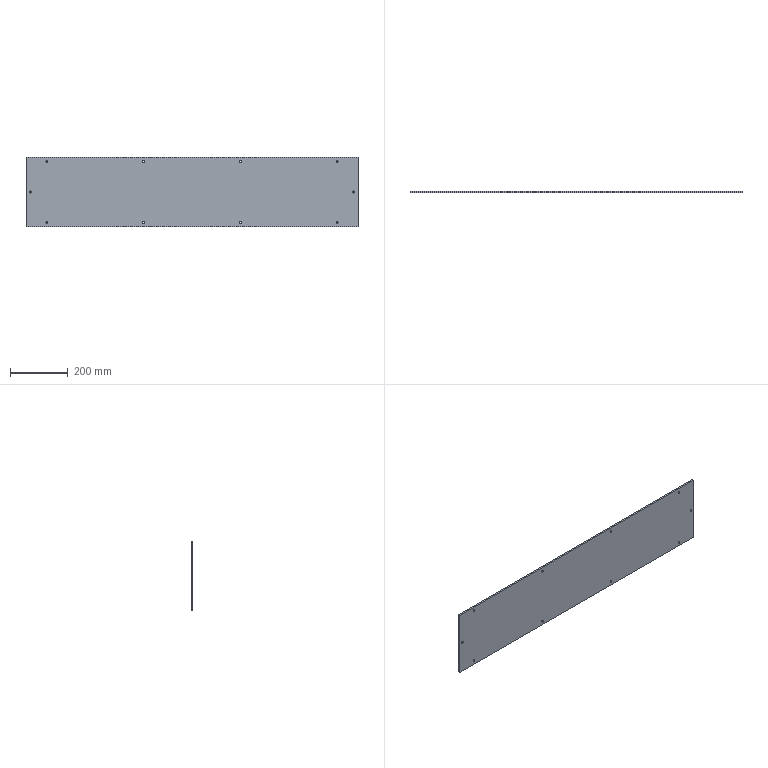Part | SolidWorks | features BaseBody 1 | 1 solid | 26 faces | box 1150 x 6 x 242 mm | volume 1667491 mm3 | cylinder 20 | plane 6 | commonest cylinder face diameters 7 x20
STEP:
#1=CARTESIAN_POINT('',(560.,0.,3.5));
#2=VERTEX_POINT('',#1);
#3=CARTESIAN_POINT('',(560.,0.,-3.5));
#4=VERTEX_POINT('',#3);
#5=CARTESIAN_POINT('',(560.,0.,0.));
#6=DIRECTION('',(0.,-1.,0.));
#7=DIRECTION('',(0.,0.,1.));
#8=AXIS2_PLACEMENT_3D('',#5,#6,#7);
#9=CIRCLE('',#8,3.5);
#10=EDGE_CURVE('',#2,#4,#9,.T.);
#11=ORIENTED_EDGE('',*,*,#10,.T.);
#12=CARTESIAN_POINT('',(560.,6.,-3.5));
#13=VERTEX_POINT('',#12);
#14=CARTESIAN_POINT('',(560.,0.,-3.5));
#15=DIRECTION('',(0.,1.,0.));
#16=VECTOR('',#15,1000.);
#17=LINE('',#14,#16);
#18=EDGE_CURVE('',#4,#13,#17,.T.);
#19=ORIENTED_EDGE('',*,*,#18,.T.);
#20=CARTESIAN_POINT('',(560.,6.,3.5));
#21=VERTEX_POINT('',#20);
#22=CARTESIAN_POINT('',(560.,6.,0.));
#23=DIRECTION('',(0.,-1.,0.));
#24=DIRECTION('',(0.,0.,1.));
#25=AXIS2_PLACEMENT_3D('',#22,#23,#24);
#26=CIRCLE('',#25,3.5);
#27=EDGE_CURVE('',#21,#13,#26,.T.);
#28=ORIENTED_EDGE('',*,*,#27,.F.);
#29=CARTESIAN_POINT('',(560.,0.,3.5));
#30=DIRECTION('',(0.,1.,0.));
#31=VECTOR('',#30,1000.);
#32=LINE('',#29,#31);
#33=EDGE_CURVE('',#2,#21,#32,.T.);
#34=ORIENTED_EDGE('',*,*,#33,.F.);
#35=EDGE_LOOP('',(#11,#19,#28,#34));
#36=FACE_OUTER_BOUND('',#35,.T.);
#37=CARTESIAN_POINT('',(560.,0.,0.));
#38=DIRECTION('',(0.,1.,0.));
#39=DIRECTION('',(0.,0.,1.));
#40=AXIS2_PLACEMENT_3D('',#37,#38,#39);
#41=CYLINDRICAL_SURFACE('',#40,3.5);
#42=ADVANCED_FACE('',(#36),#41,.F.);
#43=CARTESIAN_POINT('',(-560.,0.,-3.5));
#44=VERTEX_POINT('',#43);
#45=CARTESIAN_POINT('',(-560.,0.,3.5));
#46=VERTEX_POINT('',#45);
#47=CARTESIAN_POINT('',(-560.,0.,0.));
#48=DIRECTION('',(0.,1.,0.));
#49=DIRECTION('',(0.,0.,1.));
#50=AXIS2_PLACEMENT_3D('',#47,#48,#49);
#51=CIRCLE('',#50,3.5);
#52=EDGE_CURVE('',#44,#46,#51,.T.);
#53=ORIENTED_EDGE('',*,*,#52,.F.);
#54=CARTESIAN_POINT('',(-560.,6.,-3.5));
#55=VERTEX_POINT('',#54);
#56=CARTESIAN_POINT('',(-560.,0.,-3.5));
#57=DIRECTION('',(0.,1.,0.));
#58=VECTOR('',#57,1000.);
#59=LINE('',#56,#58);
#60=EDGE_CURVE('',#44,#55,#59,.T.);
#61=ORIENTED_EDGE('',*,*,#60,.T.);
#62=CARTESIAN_POINT('',(-560.,6.,3.5));
#63=VERTEX_POINT('',#62);
#64=CARTESIAN_POINT('',(-560.,6.,0.));
#65=DIRECTION('',(0.,1.,0.));
#66=DIRECTION('',(0.,0.,1.));
#67=AXIS2_PLACEMENT_3D('',#64,#65,#66);
#68=CIRCLE('',#67,3.5);
#69=EDGE_CURVE('',#55,#63,#68,.T.);
#70=ORIENTED_EDGE('',*,*,#69,.T.);
#71=CARTESIAN_POINT('',(-560.,0.,3.5));
#72=DIRECTION('',(0.,1.,0.));
#73=VECTOR('',#72,1000.);
#74=LINE('',#71,#73);
#75=EDGE_CURVE('',#46,#63,#74,.T.);
#76=ORIENTED_EDGE('',*,*,#75,.F.);
#77=EDGE_LOOP('',(#53,#61,#70,#76));
#78=FACE_OUTER_BOUND('',#77,.T.);
#79=CARTESIAN_POINT('',(-560.,0.,0.));
#80=DIRECTION('',(0.,1.,0.));
#81=DIRECTION('',(0.,0.,1.));
#82=AXIS2_PLACEMENT_3D('',#79,#80,#81);
#83=CYLINDRICAL_SURFACE('',#82,3.5);
#84=ADVANCED_FACE('',(#78),#83,.F.);
#85=CARTESIAN_POINT('',(502.5,0.,-109.5));
#86=VERTEX_POINT('',#85);
#87=CARTESIAN_POINT('',(502.5,0.,-102.5));
#88=VERTEX_POINT('',#87);
#89=CARTESIAN_POINT('',(502.5,0.,-106.));
#90=DIRECTION('',(0.,1.,0.));
#91=DIRECTION('',(0.,0.,1.));
#92=AXIS2_PLACEMENT_3D('',#89,#90,#91);
#93=CIRCLE('',#92,3.5);
#94=EDGE_CURVE('',#86,#88,#93,.T.);
#95=ORIENTED_EDGE('',*,*,#94,.F.);
#96=CARTESIAN_POINT('',(502.5,6.,-109.5));
#97=VERTEX_POINT('',#96);
#98=CARTESIAN_POINT('',(502.5,0.,-109.5));
#99=DIRECTION('',(0.,1.,0.));
#100=VECTOR('',#99,1000.);
#101=LINE('',#98,#100);
#102=EDGE_CURVE('',#86,#97,#101,.T.);
#103=ORIENTED_EDGE('',*,*,#102,.T.);
#104=CARTESIAN_POINT('',(502.5,6.,-102.5));
#105=VERTEX_POINT('',#104);
#106=CARTESIAN_POINT('',(502.5,6.,-106.));
#107=DIRECTION('',(0.,1.,0.));
#108=DIRECTION('',(0.,0.,1.));
#109=AXIS2_PLACEMENT_3D('',#106,#107,#108);
#110=CIRCLE('',#109,3.5);
#111=EDGE_CURVE('',#97,#105,#110,.T.);
#112=ORIENTED_EDGE('',*,*,#111,.T.);
#113=CARTESIAN_POINT('',(502.5,0.,-102.5));
#114=DIRECTION('',(0.,1.,0.));
#115=VECTOR('',#114,1000.);
#116=LINE('',#113,#115);
#117=EDGE_CURVE('',#88,#105,#116,.T.);
#118=ORIENTED_EDGE('',*,*,#117,.F.);
#119=EDGE_LOOP('',(#95,#103,#112,#118));
#120=FACE_OUTER_BOUND('',#119,.T.);
#121=CARTESIAN_POINT('',(502.5,0.,-106.));
#122=DIRECTION('',(0.,1.,0.));
#123=DIRECTION('',(0.,0.,1.));
#124=AXIS2_PLACEMENT_3D('',#121,#122,#123);
#125=CYLINDRICAL_SURFACE('',#124,3.5);
#126=ADVANCED_FACE('',(#120),#125,.F.);
#127=CARTESIAN_POINT('',(167.5,0.,-109.5));
#128=VERTEX_POINT('',#127);
#129=CARTESIAN_POINT('',(167.5,0.,-102.5));
#130=VERTEX_POINT('',#129);
#131=CARTESIAN_POINT('',(167.5,0.,-106.));
#132=DIRECTION('',(0.,1.,0.));
#133=DIRECTION('',(0.,0.,1.));
#134=AXIS2_PLACEMENT_3D('',#131,#132,#133);
#135=CIRCLE('',#134,3.5);
#136=EDGE_CURVE('',#128,#130,#135,.T.);
#137=ORIENTED_EDGE('',*,*,#136,.F.);
#138=CARTESIAN_POINT('',(167.5,6.,-109.5));
#139=VERTEX_POINT('',#138);
#140=CARTESIAN_POINT('',(167.5,0.,-109.5));
#141=DIRECTION('',(0.,1.,0.));
#142=VECTOR('',#141,1000.);
#143=LINE('',#140,#142);
#144=EDGE_CURVE('',#128,#139,#143,.T.);
#145=ORIENTED_EDGE('',*,*,#144,.T.);
#146=CARTESIAN_POINT('',(167.5,6.,-102.5));
#147=VERTEX_POINT('',#146);
#148=CARTESIAN_POINT('',(167.5,6.,-106.));
#149=DIRECTION('',(0.,1.,0.));
#150=DIRECTION('',(0.,0.,1.));
#151=AXIS2_PLACEMENT_3D('',#148,#149,#150);
#152=CIRCLE('',#151,3.5);
#153=EDGE_CURVE('',#139,#147,#152,.T.);
#154=ORIENTED_EDGE('',*,*,#153,.T.);
#155=CARTESIAN_POINT('',(167.5,0.,-102.5));
#156=DIRECTION('',(0.,1.,0.));
#157=VECTOR('',#156,1000.);
#158=LINE('',#155,#157);
#159=EDGE_CURVE('',#130,#147,#158,.T.);
#160=ORIENTED_EDGE('',*,*,#159,.F.);
#161=EDGE_LOOP('',(#137,#145,#154,#160));
#162=FACE_OUTER_BOUND('',#161,.T.);
#163=CARTESIAN_POINT('',(167.5,0.,-106.));
#164=DIRECTION('',(0.,1.,0.));
#165=DIRECTION('',(0.,0.,1.));
#166=AXIS2_PLACEMENT_3D('',#163,#164,#165);
#167=CYLINDRICAL_SURFACE('',#166,3.5);
#168=ADVANCED_FACE('',(#162),#167,.F.);
#169=CARTESIAN_POINT('',(-167.5,0.,-109.5));
#170=VERTEX_POINT('',#169);
#171=CARTESIAN_POINT('',(-167.5,0.,-102.5));
#172=VERTEX_POINT('',#171);
#173=CARTESIAN_POINT('',(-167.5,0.,-106.));
#174=DIRECTION('',(0.,1.,0.));
#175=DIRECTION('',(0.,0.,1.));
#176=AXIS2_PLACEMENT_3D('',#173,#174,#175);
#177=CIRCLE('',#176,3.5);
#178=EDGE_CURVE('',#170,#172,#177,.T.);
#179=ORIENTED_EDGE('',*,*,#178,.F.);
#180=CARTESIAN_POINT('',(-167.5,6.,-109.5));
#181=VERTEX_POINT('',#180);
#182=CARTESIAN_POINT('',(-167.5,0.,-109.5));
#183=DIRECTION('',(0.,1.,0.));
#184=VECTOR('',#183,1000.);
#185=LINE('',#182,#184);
#186=EDGE_CURVE('',#170,#181,#185,.T.);
#187=ORIENTED_EDGE('',*,*,#186,.T.);
#188=CARTESIAN_POINT('',(-167.5,6.,-102.5));
#189=VERTEX_POINT('',#188);
#190=CARTESIAN_POINT('',(-167.5,6.,-106.));
#191=DIRECTION('',(0.,1.,0.));
#192=DIRECTION('',(0.,0.,1.));
#193=AXIS2_PLACEMENT_3D('',#190,#191,#192);
#194=CIRCLE('',#193,3.5);
#195=EDGE_CURVE('',#181,#189,#194,.T.);
#196=ORIENTED_EDGE('',*,*,#195,.T.);
#197=CARTESIAN_POINT('',(-167.5,0.,-102.5));
#198=DIRECTION('',(0.,1.,0.));
#199=VECTOR('',#198,1000.);
#200=LINE('',#197,#199);
#201=EDGE_CURVE('',#172,#189,#200,.T.);
#202=ORIENTED_EDGE('',*,*,#201,.F.);
#203=EDGE_LOOP('',(#179,#187,#196,#202));
#204=FACE_OUTER_BOUND('',#203,.T.);
#205=CARTESIAN_POINT('',(-167.5,0.,-106.));
#206=DIRECTION('',(0.,1.,0.));
#207=DIRECTION('',(0.,0.,1.));
#208=AXIS2_PLACEMENT_3D('',#205,#206,#207);
#209=CYLINDRICAL_SURFACE('',#208,3.5);
#210=ADVANCED_FACE('',(#204),#209,.F.);
#211=CARTESIAN_POINT('',(502.5,0.,109.5));
#212=VERTEX_POINT('',#211);
#213=CARTESIAN_POINT('',(502.5,0.,102.5));
#214=VERTEX_POINT('',#213);
#215=CARTESIAN_POINT('',(502.5,0.,106.));
#216=DIRECTION('',(0.,-1.,0.));
#217=DIRECTION('',(0.,0.,-1.));
#218=AXIS2_PLACEMENT_3D('',#215,#216,#217);
#219=CIRCLE('',#218,3.5);
#220=EDGE_CURVE('',#212,#214,#219,.T.);
#221=ORIENTED_EDGE('',*,*,#220,.T.);
#222=CARTESIAN_POINT('',(502.5,6.,102.5));
#223=VERTEX_POINT('',#222);
#224=CARTESIAN_POINT('',(502.5,0.,102.5));
#225=DIRECTION('',(0.,1.,0.));
#226=VECTOR('',#225,1000.);
#227=LINE('',#224,#226);
#228=EDGE_CURVE('',#214,#223,#227,.T.);
#229=ORIENTED_EDGE('',*,*,#228,.T.);
#230=CARTESIAN_POINT('',(502.5,6.,109.5));
#231=VERTEX_POINT('',#230);
#232=CARTESIAN_POINT('',(502.5,6.,106.));
#233=DIRECTION('',(0.,-1.,0.));
#234=DIRECTION('',(0.,0.,-1.));
#235=AXIS2_PLACEMENT_3D('',#232,#233,#234);
#236=CIRCLE('',#235,3.5);
#237=EDGE_CURVE('',#231,#223,#236,.T.);
#238=ORIENTED_EDGE('',*,*,#237,.F.);
#239=CARTESIAN_POINT('',(502.5,0.,109.5));
#240=DIRECTION('',(0.,1.,0.));
#241=VECTOR('',#240,1000.);
#242=LINE('',#239,#241);
#243=EDGE_CURVE('',#212,#231,#242,.T.);
#244=ORIENTED_EDGE('',*,*,#243,.F.);
#245=EDGE_LOOP('',(#221,#229,#238,#244));
#246=FACE_OUTER_BOUND('',#245,.T.);
#247=CARTESIAN_POINT('',(502.5,0.,106.));
#248=DIRECTION('',(0.,1.,0.));
#249=DIRECTION('',(0.,0.,1.));
#250=AXIS2_PLACEMENT_3D('',#247,#248,#249);
#251=CYLINDRICAL_SURFACE('',#250,3.5);
#252=ADVANCED_FACE('',(#246),#251,.F.);
#253=CARTESIAN_POINT('',(167.5,0.,109.5));
#254=VERTEX_POINT('',#253);
#255=CARTESIAN_POINT('',(167.5,0.,102.5));
#256=VERTEX_POINT('',#255);
#257=CARTESIAN_POINT('',(167.5,0.,106.));
#258=DIRECTION('',(0.,-1.,0.));
#259=DIRECTION('',(0.,0.,-1.));
#260=AXIS2_PLACEMENT_3D('',#257,#258,#259);
#261=CIRCLE('',#260,3.5);
#262=EDGE_CURVE('',#254,#256,#261,.T.);
#263=ORIENTED_EDGE('',*,*,#262,.T.);
#264=CARTESIAN_POINT('',(167.5,6.,102.5));
#265=VERTEX_POINT('',#264);
#266=CARTESIAN_POINT('',(167.5,0.,102.5));
#267=DIRECTION('',(0.,1.,0.));
#268=VECTOR('',#267,1000.);
#269=LINE('',#266,#268);
#270=EDGE_CURVE('',#256,#265,#269,.T.);
#271=ORIENTED_EDGE('',*,*,#270,.T.);
#272=CARTESIAN_POINT('',(167.5,6.,109.5));
#273=VERTEX_POINT('',#272);
#274=CARTESIAN_POINT('',(167.5,6.,106.));
#275=DIRECTION('',(0.,-1.,0.));
#276=DIRECTION('',(0.,0.,-1.));
#277=AXIS2_PLACEMENT_3D('',#274,#275,#276);
#278=CIRCLE('',#277,3.5);
#279=EDGE_CURVE('',#273,#265,#278,.T.);
#280=ORIENTED_EDGE('',*,*,#279,.F.);
#281=CARTESIAN_POINT('',(167.5,0.,109.5));
#282=DIRECTION('',(0.,1.,0.));
#283=VECTOR('',#282,1000.);
#284=LINE('',#281,#283);
#285=EDGE_CURVE('',#254,#273,#284,.T.);
#286=ORIENTED_EDGE('',*,*,#285,.F.);
#287=EDGE_LOOP('',(#263,#271,#280,#286));
#288=FACE_OUTER_BOUND('',#287,.T.);
#289=CARTESIAN_POINT('',(167.5,0.,106.));
#290=DIRECTION('',(0.,1.,0.));
#291=DIRECTION('',(0.,0.,1.));
#292=AXIS2_PLACEMENT_3D('',#289,#290,#291);
#293=CYLINDRICAL_SURFACE('',#292,3.5);
#294=ADVANCED_FACE('',(#288),#293,.F.);
#295=CARTESIAN_POINT('',(-167.5,0.,109.5));
#296=VERTEX_POINT('',#295);
#297=CARTESIAN_POINT('',(-167.5,0.,102.5));
#298=VERTEX_POINT('',#297);
#299=CARTESIAN_POINT('',(-167.5,0.,106.));
#300=DIRECTION('',(0.,-1.,0.));
#301=DIRECTION('',(0.,0.,-1.));
#302=AXIS2_PLACEMENT_3D('',#299,#300,#301);
#303=CIRCLE('',#302,3.5);
#304=EDGE_CURVE('',#296,#298,#303,.T.);
#305=ORIENTED_EDGE('',*,*,#304,.T.);
#306=CARTESIAN_POINT('',(-167.5,6.,102.5));
#307=VERTEX_POINT('',#306);
#308=CARTESIAN_POINT('',(-167.5,0.,102.5));
#309=DIRECTION('',(0.,1.,0.));
#310=VECTOR('',#309,1000.);
#311=LINE('',#308,#310);
#312=EDGE_CURVE('',#298,#307,#311,.T.);
#313=ORIENTED_EDGE('',*,*,#312,.T.);
#314=CARTESIAN_POINT('',(-167.5,6.,109.5));
#315=VERTEX_POINT('',#314);
#316=CARTESIAN_POINT('',(-167.5,6.,106.));
#317=DIRECTION('',(0.,-1.,0.));
#318=DIRECTION('',(0.,0.,-1.));
#319=AXIS2_PLACEMENT_3D('',#316,#317,#318);
#320=CIRCLE('',#319,3.5);
#321=EDGE_CURVE('',#315,#307,#320,.T.);
#322=ORIENTED_EDGE('',*,*,#321,.F.);
#323=CARTESIAN_POINT('',(-167.5,0.,109.5));
#324=DIRECTION('',(0.,1.,0.));
#325=VECTOR('',#324,1000.);
#326=LINE('',#323,#325);
#327=EDGE_CURVE('',#296,#315,#326,.T.);
#328=ORIENTED_EDGE('',*,*,#327,.F.);
#329=EDGE_LOOP('',(#305,#313,#322,#328));
#330=FACE_OUTER_BOUND('',#329,.T.);
#331=CARTESIAN_POINT('',(-167.5,0.,106.));
#332=DIRECTION('',(0.,1.,0.));
#333=DIRECTION('',(0.,0.,1.));
#334=AXIS2_PLACEMENT_3D('',#331,#332,#333);
#335=CYLINDRICAL_SURFACE('',#334,3.5);
#336=ADVANCED_FACE('',(#330),#335,.F.);
#337=CARTESIAN_POINT('',(-502.5,0.,109.5));
#338=VERTEX_POINT('',#337);
#339=CARTESIAN_POINT('',(-502.5,0.,102.5));
#340=VERTEX_POINT('',#339);
#341=CARTESIAN_POINT('',(-502.5,0.,106.));
#342=DIRECTION('',(0.,-1.,0.));
#343=DIRECTION('',(0.,0.,-1.));
#344=AXIS2_PLACEMENT_3D('',#341,#342,#343);
#345=CIRCLE('',#344,3.5);
#346=EDGE_CURVE('',#338,#340,#345,.T.);
#347=ORIENTED_EDGE('',*,*,#346,.T.);
#348=CARTESIAN_POINT('',(-502.5,6.,102.5));
#349=VERTEX_POINT('',#348);
#350=CARTESIAN_POINT('',(-502.5,0.,102.5));
#351=DIRECTION('',(0.,1.,0.));
#352=VECTOR('',#351,1000.);
#353=LINE('',#350,#352);
#354=EDGE_CURVE('',#340,#349,#353,.T.);
#355=ORIENTED_EDGE('',*,*,#354,.T.);
#356=CARTESIAN_POINT('',(-502.5,6.,109.5));
#357=VERTEX_POINT('',#356);
#358=CARTESIAN_POINT('',(-502.5,6.,106.));
#359=DIRECTION('',(0.,-1.,0.));
#360=DIRECTION('',(0.,0.,-1.));
#361=AXIS2_PLACEMENT_3D('',#358,#359,#360);
#362=CIRCLE('',#361,3.5);
#363=EDGE_CURVE('',#357,#349,#362,.T.);
#364=ORIENTED_EDGE('',*,*,#363,.F.);
#365=CARTESIAN_POINT('',(-502.5,0.,109.5));
#366=DIRECTION('',(0.,1.,0.));
#367=VECTOR('',#366,1000.);
#368=LINE('',#365,#367);
#369=EDGE_CURVE('',#338,#357,#368,.T.);
#370=ORIENTED_EDGE('',*,*,#369,.F.);
#371=EDGE_LOOP('',(#347,#355,#364,#370));
#372=FACE_OUTER_BOUND('',#371,.T.);
#373=CARTESIAN_POINT('',(-502.5,0.,106.));
#374=DIRECTION('',(0.,1.,0.));
#375=DIRECTION('',(0.,0.,1.));
#376=AXIS2_PLACEMENT_3D('',#373,#374,#375);
#377=CYLINDRICAL_SURFACE('',#376,3.5);
#378=ADVANCED_FACE('',(#372),#377,.F.);
#379=CARTESIAN_POINT('',(-502.5,0.,-109.5));
#380=VERTEX_POINT('',#379);
#381=CARTESIAN_POINT('',(-502.5,0.,-102.5));
#382=VERTEX_POINT('',#381);
#383=CARTESIAN_POINT('',(-502.5,0.,-106.));
#384=DIRECTION('',(0.,1.,0.));
#385=DIRECTION('',(0.,0.,1.));
#386=AXIS2_PLACEMENT_3D('',#383,#384,#385);
#387=CIRCLE('',#386,3.5);
#388=EDGE_CURVE('',#380,#382,#387,.T.);
#389=ORIENTED_EDGE('',*,*,#388,.F.);
#390=CARTESIAN_POINT('',(-502.5,6.,-109.5));
#391=VERTEX_POINT('',#390);
#392=CARTESIAN_POINT('',(-502.5,0.,-109.5));
#393=DIRECTION('',(0.,1.,0.));
#394=VECTOR('',#393,1000.);
#395=LINE('',#392,#394);
#396=EDGE_CURVE('',#380,#391,#395,.T.);
#397=ORIENTED_EDGE('',*,*,#396,.T.);
#398=CARTESIAN_POINT('',(-502.5,6.,-102.5));
#399=VERTEX_POINT('',#398);
#400=CARTESIAN_POINT('',(-502.5,6.,-106.));
#401=DIRECTION('',(0.,1.,0.));
#402=DIRECTION('',(0.,0.,1.));
#403=AXIS2_PLACEMENT_3D('',#400,#401,#402);
#404=CIRCLE('',#403,3.5);
#405=EDGE_CURVE('',#391,#399,#404,.T.);
#406=ORIENTED_EDGE('',*,*,#405,.T.);
#407=CARTESIAN_POINT('',(-502.5,0.,-102.5));
#408=DIRECTION('',(0.,1.,0.));
#409=VECTOR('',#408,1000.);
#410=LINE('',#407,#409);
#411=EDGE_CURVE('',#382,#399,#410,.T.);
#412=ORIENTED_EDGE('',*,*,#411,.F.);
#413=EDGE_LOOP('',(#389,#397,#406,#412));
#414=FACE_OUTER_BOUND('',#413,.T.);
#415=CARTESIAN_POINT('',(-502.5,0.,-106.));
#416=DIRECTION('',(0.,1.,0.));
#417=DIRECTION('',(0.,0.,1.));
#418=AXIS2_PLACEMENT_3D('',#415,#416,#417);
#419=CYLINDRICAL_SURFACE('',#418,3.5);
#420=ADVANCED_FACE('',(#414),#419,.F.);
#421=CARTESIAN_POINT('',(-575.,0.,121.));
#422=VERTEX_POINT('',#421);
#423=CARTESIAN_POINT('',(575.,0.,121.));
#424=VERTEX_POINT('',#423);
#425=CARTESIAN_POINT('',(-575.,0.,121.));
#426=DIRECTION('',(1.,0.,0.));
#427=VECTOR('',#426,1000.);
#428=LINE('',#425,#427);
#429=EDGE_CURVE('',#422,#424,#428,.T.);
#430=ORIENTED_EDGE('',*,*,#429,.T.);
#431=CARTESIAN_POINT('',(575.,6.,121.));
#432=VERTEX_POINT('',#431);
#433=CARTESIAN_POINT('',(575.,6.,121.));
#434=DIRECTION('',(0.,-1.,0.));
#435=VECTOR('',#434,1000.);
#436=LINE('',#433,#435);
#437=EDGE_CURVE('',#432,#424,#436,.T.);
#438=ORIENTED_EDGE('',*,*,#437,.F.);
#439=CARTESIAN_POINT('',(-575.,6.,121.));
#440=VERTEX_POINT('',#439);
#441=CARTESIAN_POINT('',(-575.,6.,121.));
#442=DIRECTION('',(1.,0.,0.));
#443=VECTOR('',#442,1000.);
#444=LINE('',#441,#443);
#445=EDGE_CURVE('',#440,#432,#444,.T.);
#446=ORIENTED_EDGE('',*,*,#445,.F.);
#447=CARTESIAN_POINT('',(-575.,6.,121.));
#448=DIRECTION('',(0.,-1.,0.));
#449=VECTOR('',#448,1000.);
#450=LINE('',#447,#449);
#451=EDGE_CURVE('',#440,#422,#450,.T.);
#452=ORIENTED_EDGE('',*,*,#451,.T.);
#453=EDGE_LOOP('',(#430,#438,#446,#452));
#454=FACE_OUTER_BOUND('',#453,.T.);
#455=CARTESIAN_POINT('',(-575.,6.,121.));
#456=DIRECTION('',(0.,0.,-1.));
#457=DIRECTION('',(0.,-1.,0.));
#458=AXIS2_PLACEMENT_3D('',#455,#456,#457);
#459=PLANE('',#458);
#460=ADVANCED_FACE('',(#454),#459,.F.);
#461=CARTESIAN_POINT('',(-575.,0.,-121.));
#462=VERTEX_POINT('',#461);
#463=CARTESIAN_POINT('',(-575.,0.,121.));
#464=DIRECTION('',(0.,0.,1.));
#465=VECTOR('',#464,1000.);
#466=LINE('',#463,#465);
#467=EDGE_CURVE('',#462,#422,#466,.T.);
#468=ORIENTED_EDGE('',*,*,#467,.T.);
#469=ORIENTED_EDGE('',*,*,#451,.F.);
#470=CARTESIAN_POINT('',(-575.,6.,-121.));
#471=VERTEX_POINT('',#470);
#472=CARTESIAN_POINT('',(-575.,6.,121.));
#473=DIRECTION('',(0.,0.,1.));
#474=VECTOR('',#473,1000.);
#475=LINE('',#472,#474);
#476=EDGE_CURVE('',#471,#440,#475,.T.);
#477=ORIENTED_EDGE('',*,*,#476,.F.);
#478=CARTESIAN_POINT('',(-575.,6.,-121.));
#479=DIRECTION('',(0.,-1.,0.));
#480=VECTOR('',#479,1000.);
#481=LINE('',#478,#480);
#482=EDGE_CURVE('',#471,#462,#481,.T.);
#483=ORIENTED_EDGE('',*,*,#482,.T.);
#484=EDGE_LOOP('',(#468,#469,#477,#483));
#485=FACE_OUTER_BOUND('',#484,.T.);
#486=CARTESIAN_POINT('',(-575.,6.,121.));
#487=DIRECTION('',(1.,0.,0.));
#488=DIRECTION('',(0.,1.,0.));
#489=AXIS2_PLACEMENT_3D('',#486,#487,#488);
#490=PLANE('',#489);
#491=ADVANCED_FACE('',(#485),#490,.F.);
#492=CARTESIAN_POINT('',(575.,0.,-121.));
#493=VERTEX_POINT('',#492);
#494=CARTESIAN_POINT('',(-575.,0.,-121.));
#495=DIRECTION('',(-1.,0.,0.));
#496=VECTOR('',#495,1000.);
#497=LINE('',#494,#496);
#498=EDGE_CURVE('',#493,#462,#497,.T.);
#499=ORIENTED_EDGE('',*,*,#498,.T.);
#500=ORIENTED_EDGE('',*,*,#482,.F.);
#501=CARTESIAN_POINT('',(575.,6.,-121.));
#502=VERTEX_POINT('',#501);
#503=CARTESIAN_POINT('',(-575.,6.,-121.));
#504=DIRECTION('',(-1.,0.,0.));
#505=VECTOR('',#504,1000.);
#506=LINE('',#503,#505);
#507=EDGE_CURVE('',#502,#471,#506,.T.);
#508=ORIENTED_EDGE('',*,*,#507,.F.);
#509=CARTESIAN_POINT('',(575.,6.,-121.));
#510=DIRECTION('',(0.,-1.,0.));
#511=VECTOR('',#510,1000.);
#512=LINE('',#509,#511);
#513=EDGE_CURVE('',#502,#493,#512,.T.);
#514=ORIENTED_EDGE('',*,*,#513,.T.);
#515=EDGE_LOOP('',(#499,#500,#508,#514));
#516=FACE_OUTER_BOUND('',#515,.T.);
#517=CARTESIAN_POINT('',(-575.,6.,-121.));
#518=DIRECTION('',(0.,0.,1.));
#519=DIRECTION('',(1.,0.,0.));
#520=AXIS2_PLACEMENT_3D('',#517,#518,#519);
#521=PLANE('',#520);
#522=ADVANCED_FACE('',(#516),#521,.F.);
#523=CARTESIAN_POINT('',(575.,0.,121.));
#524=DIRECTION('',(0.,0.,-1.));
#525=VECTOR('',#524,1000.);
#526=LINE('',#523,#525);
#527=EDGE_CURVE('',#424,#493,#526,.T.);
#528=ORIENTED_EDGE('',*,*,#527,.T.);
#529=ORIENTED_EDGE('',*,*,#513,.F.);
#530=CARTESIAN_POINT('',(575.,6.,121.));
#531=DIRECTION('',(0.,0.,-1.));
#532=VECTOR('',#531,1000.);
#533=LINE('',#530,#532);
#534=EDGE_CURVE('',#432,#502,#533,.T.);
#535=ORIENTED_EDGE('',*,*,#534,.F.);
#536=ORIENTED_EDGE('',*,*,#437,.T.);
#537=EDGE_LOOP('',(#528,#529,#535,#536));
#538=FACE_OUTER_BOUND('',#537,.T.);
#539=CARTESIAN_POINT('',(575.,6.,121.));
#540=DIRECTION('',(-1.,0.,0.));
#541=DIRECTION('',(0.,0.,1.));
#542=AXIS2_PLACEMENT_3D('',#539,#540,#541);
#543=PLANE('',#542);
#544=ADVANCED_FACE('',(#538),#543,.F.);
#545=ORIENTED_EDGE('',*,*,#10,.F.);
#546=CARTESIAN_POINT('',(560.,0.,0.));
#547=DIRECTION('',(0.,-1.,0.));
#548=DIRECTION('',(0.,0.,1.));
#549=AXIS2_PLACEMENT_3D('',#546,#547,#548);
#550=CIRCLE('',#549,3.5);
#551=EDGE_CURVE('',#4,#2,#550,.T.);
#552=ORIENTED_EDGE('',*,*,#551,.F.);
#553=EDGE_LOOP('',(#545,#552));
#554=FACE_BOUND('',#553,.T.);
#555=CARTESIAN_POINT('',(-560.,0.,0.));
#556=DIRECTION('',(0.,1.,0.));
#557=DIRECTION('',(0.,0.,1.));
#558=AXIS2_PLACEMENT_3D('',#555,#556,#557);
#559=CIRCLE('',#558,3.5);
#560=EDGE_CURVE('',#46,#44,#559,.T.);
#561=ORIENTED_EDGE('',*,*,#560,.T.);
#562=ORIENTED_EDGE('',*,*,#52,.T.);
#563=EDGE_LOOP('',(#561,#562));
#564=FACE_BOUND('',#563,.T.);
#565=CARTESIAN_POINT('',(-167.5,0.,-106.));
#566=DIRECTION('',(0.,1.,0.));
#567=DIRECTION('',(0.,0.,1.));
#568=AXIS2_PLACEMENT_3D('',#565,#566,#567);
#569=CIRCLE('',#568,3.5);
#570=EDGE_CURVE('',#172,#170,#569,.T.);
#571=ORIENTED_EDGE('',*,*,#570,.T.);
#572=ORIENTED_EDGE('',*,*,#178,.T.);
#573=EDGE_LOOP('',(#571,#572));
#574=FACE_BOUND('',#573,.T.);
#575=ORIENTED_EDGE('',*,*,#262,.F.);
#576=CARTESIAN_POINT('',(167.5,0.,106.));
#577=DIRECTION('',(0.,-1.,0.));
#578=DIRECTION('',(0.,0.,-1.));
#579=AXIS2_PLACEMENT_3D('',#576,#577,#578);
#580=CIRCLE('',#579,3.5);
#581=EDGE_CURVE('',#256,#254,#580,.T.);
#582=ORIENTED_EDGE('',*,*,#581,.F.);
#583=EDGE_LOOP('',(#575,#582));
#584=FACE_BOUND('',#583,.T.);
#585=ORIENTED_EDGE('',*,*,#346,.F.);
#586=CARTESIAN_POINT('',(-502.5,0.,106.));
#587=DIRECTION('',(0.,-1.,0.));
#588=DIRECTION('',(0.,0.,-1.));
#589=AXIS2_PLACEMENT_3D('',#586,#587,#588);
#590=CIRCLE('',#589,3.5);
#591=EDGE_CURVE('',#340,#338,#590,.T.);
#592=ORIENTED_EDGE('',*,*,#591,.F.);
#593=EDGE_LOOP('',(#585,#592));
#594=FACE_BOUND('',#593,.T.);
#595=CARTESIAN_POINT('',(-502.5,0.,-106.));
#596=DIRECTION('',(0.,1.,0.));
#597=DIRECTION('',(0.,0.,1.));
#598=AXIS2_PLACEMENT_3D('',#595,#596,#597);
#599=CIRCLE('',#598,3.5);
#600=EDGE_CURVE('',#382,#380,#599,.T.);
#601=ORIENTED_EDGE('',*,*,#600,.T.);
#602=ORIENTED_EDGE('',*,*,#388,.T.);
#603=EDGE_LOOP('',(#601,#602));
#604=FACE_BOUND('',#603,.T.);
#605=ORIENTED_EDGE('',*,*,#304,.F.);
#606=CARTESIAN_POINT('',(-167.5,0.,106.));
#607=DIRECTION('',(0.,-1.,0.));
#608=DIRECTION('',(0.,0.,-1.));
#609=AXIS2_PLACEMENT_3D('',#606,#607,#608);
#610=CIRCLE('',#609,3.5);
#611=EDGE_CURVE('',#298,#296,#610,.T.);
#612=ORIENTED_EDGE('',*,*,#611,.F.);
#613=EDGE_LOOP('',(#605,#612));
#614=FACE_BOUND('',#613,.T.);
#615=ORIENTED_EDGE('',*,*,#220,.F.);
#616=CARTESIAN_POINT('',(502.5,0.,106.));
#617=DIRECTION('',(0.,-1.,0.));
#618=DIRECTION('',(0.,0.,-1.));
#619=AXIS2_PLACEMENT_3D('',#616,#617,#618);
#620=CIRCLE('',#619,3.5);
#621=EDGE_CURVE('',#214,#212,#620,.T.);
#622=ORIENTED_EDGE('',*,*,#621,.F.);
#623=EDGE_LOOP('',(#615,#622));
#624=FACE_BOUND('',#623,.T.);
#625=CARTESIAN_POINT('',(167.5,0.,-106.));
#626=DIRECTION('',(0.,1.,0.));
#627=DIRECTION('',(0.,0.,1.));
#628=AXIS2_PLACEMENT_3D('',#625,#626,#627);
#629=CIRCLE('',#628,3.5);
#630=EDGE_CURVE('',#130,#128,#629,.T.);
#631=ORIENTED_EDGE('',*,*,#630,.T.);
#632=ORIENTED_EDGE('',*,*,#136,.T.);
#633=EDGE_LOOP('',(#631,#632));
#634=FACE_BOUND('',#633,.T.);
#635=CARTESIAN_POINT('',(502.5,0.,-106.));
#636=DIRECTION('',(0.,1.,0.));
#637=DIRECTION('',(0.,0.,1.));
#638=AXIS2_PLACEMENT_3D('',#635,#636,#637);
#639=CIRCLE('',#638,3.5);
#640=EDGE_CURVE('',#88,#86,#639,.T.);
#641=ORIENTED_EDGE('',*,*,#640,.T.);
#642=ORIENTED_EDGE('',*,*,#94,.T.);
#643=EDGE_LOOP('',(#641,#642));
#644=FACE_BOUND('',#643,.T.);
#645=ORIENTED_EDGE('',*,*,#527,.F.);
#646=ORIENTED_EDGE('',*,*,#429,.F.);
#647=ORIENTED_EDGE('',*,*,#467,.F.);
#648=ORIENTED_EDGE('',*,*,#498,.F.);
#649=EDGE_LOOP('',(#645,#646,#647,#648));
#650=FACE_OUTER_BOUND('',#649,.T.);
#651=CARTESIAN_POINT('',(0.,0.,0.));
#652=DIRECTION('',(0.,-1.,0.));
#653=DIRECTION('',(0.,0.,-1.));
#654=AXIS2_PLACEMENT_3D('',#651,#652,#653);
#655=PLANE('',#654);
#656=ADVANCED_FACE('',(#554,#564,#574,#584,#594,#604,#614,#624,#634,#644,#650),#655,.T.);
#657=ORIENTED_EDGE('',*,*,#27,.T.);
#658=CARTESIAN_POINT('',(560.,6.,0.));
#659=DIRECTION('',(0.,-1.,0.));
#660=DIRECTION('',(0.,0.,1.));
#661=AXIS2_PLACEMENT_3D('',#658,#659,#660);
#662=CIRCLE('',#661,3.5);
#663=EDGE_CURVE('',#13,#21,#662,.T.);
#664=ORIENTED_EDGE('',*,*,#663,.T.);
#665=EDGE_LOOP('',(#657,#664));
#666=FACE_BOUND('',#665,.T.);
#667=CARTESIAN_POINT('',(-560.,6.,0.));
#668=DIRECTION('',(0.,1.,0.));
#669=DIRECTION('',(0.,0.,1.));
#670=AXIS2_PLACEMENT_3D('',#667,#668,#669);
#671=CIRCLE('',#670,3.5);
#672=EDGE_CURVE('',#63,#55,#671,.T.);
#673=ORIENTED_EDGE('',*,*,#672,.F.);
#674=ORIENTED_EDGE('',*,*,#69,.F.);
#675=EDGE_LOOP('',(#673,#674));
#676=FACE_BOUND('',#675,.T.);
#677=CARTESIAN_POINT('',(-167.5,6.,-106.));
#678=DIRECTION('',(0.,1.,0.));
#679=DIRECTION('',(0.,0.,1.));
#680=AXIS2_PLACEMENT_3D('',#677,#678,#679);
#681=CIRCLE('',#680,3.5);
#682=EDGE_CURVE('',#189,#181,#681,.T.);
#683=ORIENTED_EDGE('',*,*,#682,.F.);
#684=ORIENTED_EDGE('',*,*,#195,.F.);
#685=EDGE_LOOP('',(#683,#684));
#686=FACE_BOUND('',#685,.T.);
#687=ORIENTED_EDGE('',*,*,#279,.T.);
#688=CARTESIAN_POINT('',(167.5,6.,106.));
#689=DIRECTION('',(0.,-1.,0.));
#690=DIRECTION('',(0.,0.,-1.));
#691=AXIS2_PLACEMENT_3D('',#688,#689,#690);
#692=CIRCLE('',#691,3.5);
#693=EDGE_CURVE('',#265,#273,#692,.T.);
#694=ORIENTED_EDGE('',*,*,#693,.T.);
#695=EDGE_LOOP('',(#687,#694));
#696=FACE_BOUND('',#695,.T.);
#697=ORIENTED_EDGE('',*,*,#363,.T.);
#698=CARTESIAN_POINT('',(-502.5,6.,106.));
#699=DIRECTION('',(0.,-1.,0.));
#700=DIRECTION('',(0.,0.,-1.));
#701=AXIS2_PLACEMENT_3D('',#698,#699,#700);
#702=CIRCLE('',#701,3.5);
#703=EDGE_CURVE('',#349,#357,#702,.T.);
#704=ORIENTED_EDGE('',*,*,#703,.T.);
#705=EDGE_LOOP('',(#697,#704));
#706=FACE_BOUND('',#705,.T.);
#707=CARTESIAN_POINT('',(-502.5,6.,-106.));
#708=DIRECTION('',(0.,1.,0.));
#709=DIRECTION('',(0.,0.,1.));
#710=AXIS2_PLACEMENT_3D('',#707,#708,#709);
#711=CIRCLE('',#710,3.5);
#712=EDGE_CURVE('',#399,#391,#711,.T.);
#713=ORIENTED_EDGE('',*,*,#712,.F.);
#714=ORIENTED_EDGE('',*,*,#405,.F.);
#715=EDGE_LOOP('',(#713,#714));
#716=FACE_BOUND('',#715,.T.);
#717=ORIENTED_EDGE('',*,*,#321,.T.);
#718=CARTESIAN_POINT('',(-167.5,6.,106.));
#719=DIRECTION('',(0.,-1.,0.));
#720=DIRECTION('',(0.,0.,-1.));
#721=AXIS2_PLACEMENT_3D('',#718,#719,#720);
#722=CIRCLE('',#721,3.5);
#723=EDGE_CURVE('',#307,#315,#722,.T.);
#724=ORIENTED_EDGE('',*,*,#723,.T.);
#725=EDGE_LOOP('',(#717,#724));
#726=FACE_BOUND('',#725,.T.);
#727=ORIENTED_EDGE('',*,*,#237,.T.);
#728=CARTESIAN_POINT('',(502.5,6.,106.));
#729=DIRECTION('',(0.,-1.,0.));
#730=DIRECTION('',(0.,0.,-1.));
#731=AXIS2_PLACEMENT_3D('',#728,#729,#730);
#732=CIRCLE('',#731,3.5);
#733=EDGE_CURVE('',#223,#231,#732,.T.);
#734=ORIENTED_EDGE('',*,*,#733,.T.);
#735=EDGE_LOOP('',(#727,#734));
#736=FACE_BOUND('',#735,.T.);
#737=CARTESIAN_POINT('',(167.5,6.,-106.));
#738=DIRECTION('',(0.,1.,0.));
#739=DIRECTION('',(0.,0.,1.));
#740=AXIS2_PLACEMENT_3D('',#737,#738,#739);
#741=CIRCLE('',#740,3.5);
#742=EDGE_CURVE('',#147,#139,#741,.T.);
#743=ORIENTED_EDGE('',*,*,#742,.F.);
#744=ORIENTED_EDGE('',*,*,#153,.F.);
#745=EDGE_LOOP('',(#743,#744));
#746=FACE_BOUND('',#745,.T.);
#747=CARTESIAN_POINT('',(502.5,6.,-106.));
#748=DIRECTION('',(0.,1.,0.));
#749=DIRECTION('',(0.,0.,1.));
#750=AXIS2_PLACEMENT_3D('',#747,#748,#749);
#751=CIRCLE('',#750,3.5);
#752=EDGE_CURVE('',#105,#97,#751,.T.);
#753=ORIENTED_EDGE('',*,*,#752,.F.);
#754=ORIENTED_EDGE('',*,*,#111,.F.);
#755=EDGE_LOOP('',(#753,#754));
#756=FACE_BOUND('',#755,.T.);
#757=ORIENTED_EDGE('',*,*,#534,.T.);
#758=ORIENTED_EDGE('',*,*,#507,.T.);
#759=ORIENTED_EDGE('',*,*,#476,.T.);
#760=ORIENTED_EDGE('',*,*,#445,.T.);
#761=EDGE_LOOP('',(#757,#758,#759,#760));
#762=FACE_OUTER_BOUND('',#761,.T.);
#763=CARTESIAN_POINT('',(0.,6.,0.));
#764=DIRECTION('',(0.,-1.,0.));
#765=DIRECTION('',(0.,0.,-1.));
#766=AXIS2_PLACEMENT_3D('',#763,#764,#765);
#767=PLANE('',#766);
#768=ADVANCED_FACE('',(#666,#676,#686,#696,#706,#716,#726,#736,#746,#756,#762),#767,.F.);
#769=ORIENTED_EDGE('',*,*,#396,.F.);
#770=ORIENTED_EDGE('',*,*,#600,.F.);
#771=ORIENTED_EDGE('',*,*,#411,.T.);
#772=ORIENTED_EDGE('',*,*,#712,.T.);
#773=EDGE_LOOP('',(#769,#770,#771,#772));
#774=FACE_OUTER_BOUND('',#773,.T.);
#775=CARTESIAN_POINT('',(-502.5,0.,-106.));
#776=DIRECTION('',(0.,1.,0.));
#777=DIRECTION('',(0.,0.,1.));
#778=AXIS2_PLACEMENT_3D('',#775,#776,#777);
#779=CYLINDRICAL_SURFACE('',#778,3.5);
#780=ADVANCED_FACE('',(#774),#779,.F.);
#781=ORIENTED_EDGE('',*,*,#354,.F.);
#782=ORIENTED_EDGE('',*,*,#591,.T.);
#783=ORIENTED_EDGE('',*,*,#369,.T.);
#784=ORIENTED_EDGE('',*,*,#703,.F.);
#785=EDGE_LOOP('',(#781,#782,#783,#784));
#786=FACE_OUTER_BOUND('',#785,.T.);
#787=CARTESIAN_POINT('',(-502.5,0.,106.));
#788=DIRECTION('',(0.,1.,0.));
#789=DIRECTION('',(0.,0.,1.));
#790=AXIS2_PLACEMENT_3D('',#787,#788,#789);
#791=CYLINDRICAL_SURFACE('',#790,3.5);
#792=ADVANCED_FACE('',(#786),#791,.F.);
#793=ORIENTED_EDGE('',*,*,#312,.F.);
#794=ORIENTED_EDGE('',*,*,#611,.T.);
#795=ORIENTED_EDGE('',*,*,#327,.T.);
#796=ORIENTED_EDGE('',*,*,#723,.F.);
#797=EDGE_LOOP('',(#793,#794,#795,#796));
#798=FACE_OUTER_BOUND('',#797,.T.);
#799=CARTESIAN_POINT('',(-167.5,0.,106.));
#800=DIRECTION('',(0.,1.,0.));
#801=DIRECTION('',(0.,0.,1.));
#802=AXIS2_PLACEMENT_3D('',#799,#800,#801);
#803=CYLINDRICAL_SURFACE('',#802,3.5);
#804=ADVANCED_FACE('',(#798),#803,.F.);
#805=ORIENTED_EDGE('',*,*,#270,.F.);
#806=ORIENTED_EDGE('',*,*,#581,.T.);
#807=ORIENTED_EDGE('',*,*,#285,.T.);
#808=ORIENTED_EDGE('',*,*,#693,.F.);
#809=EDGE_LOOP('',(#805,#806,#807,#808));
#810=FACE_OUTER_BOUND('',#809,.T.);
#811=CARTESIAN_POINT('',(167.5,0.,106.));
#812=DIRECTION('',(0.,1.,0.));
#813=DIRECTION('',(0.,0.,1.));
#814=AXIS2_PLACEMENT_3D('',#811,#812,#813);
#815=CYLINDRICAL_SURFACE('',#814,3.5);
#816=ADVANCED_FACE('',(#810),#815,.F.);
#817=ORIENTED_EDGE('',*,*,#228,.F.);
#818=ORIENTED_EDGE('',*,*,#621,.T.);
#819=ORIENTED_EDGE('',*,*,#243,.T.);
#820=ORIENTED_EDGE('',*,*,#733,.F.);
#821=EDGE_LOOP('',(#817,#818,#819,#820));
#822=FACE_OUTER_BOUND('',#821,.T.);
#823=CARTESIAN_POINT('',(502.5,0.,106.));
#824=DIRECTION('',(0.,1.,0.));
#825=DIRECTION('',(0.,0.,1.));
#826=AXIS2_PLACEMENT_3D('',#823,#824,#825);
#827=CYLINDRICAL_SURFACE('',#826,3.5);
#828=ADVANCED_FACE('',(#822),#827,.F.);
#829=ORIENTED_EDGE('',*,*,#186,.F.);
#830=ORIENTED_EDGE('',*,*,#570,.F.);
#831=ORIENTED_EDGE('',*,*,#201,.T.);
#832=ORIENTED_EDGE('',*,*,#682,.T.);
#833=EDGE_LOOP('',(#829,#830,#831,#832));
#834=FACE_OUTER_BOUND('',#833,.T.);
#835=CARTESIAN_POINT('',(-167.5,0.,-106.));
#836=DIRECTION('',(0.,1.,0.));
#837=DIRECTION('',(0.,0.,1.));
#838=AXIS2_PLACEMENT_3D('',#835,#836,#837);
#839=CYLINDRICAL_SURFACE('',#838,3.5);
#840=ADVANCED_FACE('',(#834),#839,.F.);
#841=ORIENTED_EDGE('',*,*,#144,.F.);
#842=ORIENTED_EDGE('',*,*,#630,.F.);
#843=ORIENTED_EDGE('',*,*,#159,.T.);
#844=ORIENTED_EDGE('',*,*,#742,.T.);
#845=EDGE_LOOP('',(#841,#842,#843,#844));
#846=FACE_OUTER_BOUND('',#845,.T.);
#847=CARTESIAN_POINT('',(167.5,0.,-106.));
#848=DIRECTION('',(0.,1.,0.));
#849=DIRECTION('',(0.,0.,1.));
#850=AXIS2_PLACEMENT_3D('',#847,#848,#849);
#851=CYLINDRICAL_SURFACE('',#850,3.5);
#852=ADVANCED_FACE('',(#846),#851,.F.);
#853=ORIENTED_EDGE('',*,*,#102,.F.);
#854=ORIENTED_EDGE('',*,*,#640,.F.);
#855=ORIENTED_EDGE('',*,*,#117,.T.);
#856=ORIENTED_EDGE('',*,*,#752,.T.);
#857=EDGE_LOOP('',(#853,#854,#855,#856));
#858=FACE_OUTER_BOUND('',#857,.T.);
#859=CARTESIAN_POINT('',(502.5,0.,-106.));
#860=DIRECTION('',(0.,1.,0.));
#861=DIRECTION('',(0.,0.,1.));
#862=AXIS2_PLACEMENT_3D('',#859,#860,#861);
#863=CYLINDRICAL_SURFACE('',#862,3.5);
#864=ADVANCED_FACE('',(#858),#863,.F.);
#865=ORIENTED_EDGE('',*,*,#60,.F.);
#866=ORIENTED_EDGE('',*,*,#560,.F.);
#867=ORIENTED_EDGE('',*,*,#75,.T.);
#868=ORIENTED_EDGE('',*,*,#672,.T.);
#869=EDGE_LOOP('',(#865,#866,#867,#868));
#870=FACE_OUTER_BOUND('',#869,.T.);
#871=CARTESIAN_POINT('',(-560.,0.,0.));
#872=DIRECTION('',(0.,1.,0.));
#873=DIRECTION('',(0.,0.,1.));
#874=AXIS2_PLACEMENT_3D('',#871,#872,#873);
#875=CYLINDRICAL_SURFACE('',#874,3.5);
#876=ADVANCED_FACE('',(#870),#875,.F.);
#877=ORIENTED_EDGE('',*,*,#18,.F.);
#878=ORIENTED_EDGE('',*,*,#551,.T.);
#879=ORIENTED_EDGE('',*,*,#33,.T.);
#880=ORIENTED_EDGE('',*,*,#663,.F.);
#881=EDGE_LOOP('',(#877,#878,#879,#880));
#882=FACE_OUTER_BOUND('',#881,.T.);
#883=CARTESIAN_POINT('',(560.,0.,0.));
#884=DIRECTION('',(0.,1.,0.));
#885=DIRECTION('',(0.,0.,1.));
#886=AXIS2_PLACEMENT_3D('',#883,#884,#885);
#887=CYLINDRICAL_SURFACE('',#886,3.5);
#888=ADVANCED_FACE('',(#882),#887,.F.);
#889=CLOSED_SHELL('',(#42,#84,#126,#168,#210,#252,#294,#336,#378,#420,#460,#491,#522,#544,#656,#768,#780,#792,#804,#816,#828,#840,#852,#864,#876,#888));
#890=MANIFOLD_SOLID_BREP('',#889);
#891=CARTESIAN_POINT('',(0.,0.,0.));
#892=DIRECTION('',(0.,0.,1.));
#893=DIRECTION('',(1.,0.,0.));
#894=AXIS2_PLACEMENT_3D('',#891,#892,#893);
#895=(LENGTH_UNIT()NAMED_UNIT(*)SI_UNIT(.MILLI.,.METRE.));
#896=UNCERTAINTY_MEASURE_WITH_UNIT(LENGTH_MEASURE(0.00001),#895,'','');
#897=(NAMED_UNIT(*)PLANE_ANGLE_UNIT()SI_UNIT($,.RADIAN.));
#898=(NAMED_UNIT(*)SI_UNIT($,.STERADIAN.)SOLID_ANGLE_UNIT());
#899=(GEOMETRIC_REPRESENTATION_CONTEXT(3)GLOBAL_UNCERTAINTY_ASSIGNED_CONTEXT((#896))GLOBAL_UNIT_ASSIGNED_CONTEXT((#895,#897,#898))REPRESENTATION_CONTEXT('',''));
#900=ADVANCED_BREP_SHAPE_REPRESENTATION('',(#890,#894),#899);